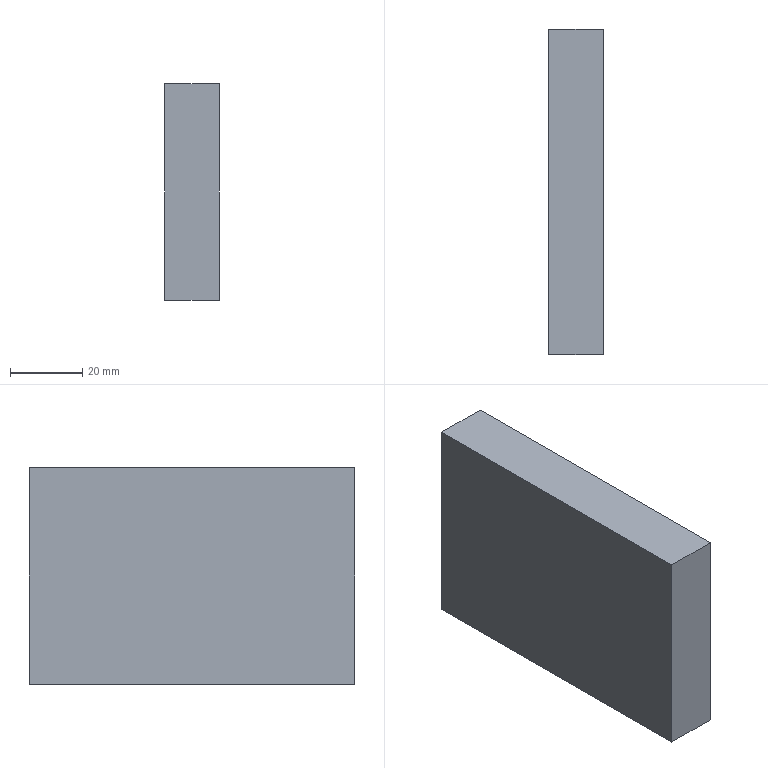Part | STEP file | Tube necking machine_id574_x_t | 1 solid | 6 faces | box 15 x 90 x 60 mm | volume 81000 mm3 | plane 6
STEP:
#1=CARTESIAN_POINT('',(0.,0.,0.));
#2=DIRECTION('',(0.,0.,1.));
#3=DIRECTION('',(1.,0.,0.));
#4=AXIS2_PLACEMENT_3D('',#1,#2,#3);
#5=CARTESIAN_POINT('',(235.5,5.,216.));
#6=VERTEX_POINT('',#5);
#7=CARTESIAN_POINT('',(250.5,5.,216.));
#8=VERTEX_POINT('',#7);
#9=CARTESIAN_POINT('',(235.5,5.,216.));
#10=DIRECTION('',(1.,0.,0.));
#11=VECTOR('',#10,1.);
#12=LINE('',#9,#11);
#13=CARTESIAN_POINT('',(8.,0.,216.));
#14=DIRECTION('',(0.,0.,1.));
#15=DIRECTION('',(1.,0.,0.));
#16=AXIS2_PLACEMENT_3D('',#13,#14,#15);
#17=PLANE('',#16);
#18=CARTESIAN_POINT('',(227.5,5.));
#19=DIRECTION('',(1.,0.));
#20=VECTOR('',#19,1.);
#21=LINE('',#18,#20);
#22=(GEOMETRIC_REPRESENTATION_CONTEXT(2)PARAMETRIC_REPRESENTATION_CONTEXT()REPRESENTATION_CONTEXT('',''));
#23=DEFINITIONAL_REPRESENTATION('',(#21),#22);
#24=PCURVE('',#17,#23);
#25=CARTESIAN_POINT('',(235.5,5.,252.));
#26=DIRECTION('',(0.,1.,0.));
#27=DIRECTION('',(0.,0.,1.));
#28=AXIS2_PLACEMENT_3D('',#25,#26,#27);
#29=PLANE('',#28);
#30=CARTESIAN_POINT('',(-36.,0.));
#31=DIRECTION('',(0.,1.));
#32=VECTOR('',#31,1.);
#33=LINE('',#30,#32);
#34=(GEOMETRIC_REPRESENTATION_CONTEXT(2)PARAMETRIC_REPRESENTATION_CONTEXT()REPRESENTATION_CONTEXT('',''));
#35=DEFINITIONAL_REPRESENTATION('',(#33),#34);
#36=PCURVE('',#29,#35);
#37=SURFACE_CURVE('',#12,(#24,#36),.PCURVE_S1.);
#38=EDGE_CURVE('',#6,#8,#37,.T.);
#39=ORIENTED_EDGE('',*,*,#38,.T.);
#40=CARTESIAN_POINT('',(250.5,95.,216.));
#41=VERTEX_POINT('',#40);
#42=CARTESIAN_POINT('',(250.5,0.,216.));
#43=DIRECTION('',(0.,-1.,0.));
#44=VECTOR('',#43,1.);
#45=LINE('',#42,#44);
#46=CARTESIAN_POINT('',(242.5,0.));
#47=DIRECTION('',(0.,-1.));
#48=VECTOR('',#47,1.);
#49=LINE('',#46,#48);
#50=(GEOMETRIC_REPRESENTATION_CONTEXT(2)PARAMETRIC_REPRESENTATION_CONTEXT()REPRESENTATION_CONTEXT('',''));
#51=DEFINITIONAL_REPRESENTATION('',(#49),#50);
#52=PCURVE('',#17,#51);
#53=CARTESIAN_POINT('',(250.5,80.,332.));
#54=DIRECTION('',(1.,0.,0.));
#55=DIRECTION('',(0.,0.,-1.));
#56=AXIS2_PLACEMENT_3D('',#53,#54,#55);
#57=PLANE('',#56);
#58=CARTESIAN_POINT('',(116.,-80.));
#59=DIRECTION('',(0.,-1.));
#60=VECTOR('',#59,1.);
#61=LINE('',#58,#60);
#62=(GEOMETRIC_REPRESENTATION_CONTEXT(2)PARAMETRIC_REPRESENTATION_CONTEXT()REPRESENTATION_CONTEXT('',''));
#63=DEFINITIONAL_REPRESENTATION('',(#61),#62);
#64=PCURVE('',#57,#63);
#65=SURFACE_CURVE('',#45,(#52,#64),.PCURVE_S1.);
#66=EDGE_CURVE('',#41,#8,#65,.T.);
#67=ORIENTED_EDGE('',*,*,#66,.F.);
#68=CARTESIAN_POINT('',(235.5,95.,216.));
#69=VERTEX_POINT('',#68);
#70=CARTESIAN_POINT('',(305.5,95.,216.));
#71=DIRECTION('',(-1.,0.,0.));
#72=VECTOR('',#71,1.);
#73=LINE('',#70,#72);
#74=CARTESIAN_POINT('',(297.5,95.));
#75=DIRECTION('',(-1.,0.));
#76=VECTOR('',#75,1.);
#77=LINE('',#74,#76);
#78=(GEOMETRIC_REPRESENTATION_CONTEXT(2)PARAMETRIC_REPRESENTATION_CONTEXT()REPRESENTATION_CONTEXT('',''));
#79=DEFINITIONAL_REPRESENTATION('',(#77),#78);
#80=PCURVE('',#17,#79);
#81=CARTESIAN_POINT('',(305.5,95.,252.));
#82=DIRECTION('',(0.,-1.,0.));
#83=DIRECTION('',(0.,0.,-1.));
#84=AXIS2_PLACEMENT_3D('',#81,#82,#83);
#85=PLANE('',#84);
#86=CARTESIAN_POINT('',(36.,0.));
#87=DIRECTION('',(0.,-1.));
#88=VECTOR('',#87,1.);
#89=LINE('',#86,#88);
#90=(GEOMETRIC_REPRESENTATION_CONTEXT(2)PARAMETRIC_REPRESENTATION_CONTEXT()REPRESENTATION_CONTEXT('',''));
#91=DEFINITIONAL_REPRESENTATION('',(#89),#90);
#92=PCURVE('',#85,#91);
#93=SURFACE_CURVE('',#73,(#80,#92),.PCURVE_S1.);
#94=EDGE_CURVE('',#41,#69,#93,.T.);
#95=ORIENTED_EDGE('',*,*,#94,.T.);
#96=CARTESIAN_POINT('',(235.5,95.,216.));
#97=DIRECTION('',(0.,-1.,0.));
#98=VECTOR('',#97,1.);
#99=LINE('',#96,#98);
#100=CARTESIAN_POINT('',(227.5,95.));
#101=DIRECTION('',(0.,-1.));
#102=VECTOR('',#101,1.);
#103=LINE('',#100,#102);
#104=(GEOMETRIC_REPRESENTATION_CONTEXT(2)PARAMETRIC_REPRESENTATION_CONTEXT()REPRESENTATION_CONTEXT('',''));
#105=DEFINITIONAL_REPRESENTATION('',(#103),#104);
#106=PCURVE('',#17,#105);
#107=CARTESIAN_POINT('',(235.5,95.,252.));
#108=DIRECTION('',(1.,0.,0.));
#109=DIRECTION('',(0.,0.,-1.));
#110=AXIS2_PLACEMENT_3D('',#107,#108,#109);
#111=PLANE('',#110);
#112=CARTESIAN_POINT('',(36.,0.));
#113=DIRECTION('',(0.,-1.));
#114=VECTOR('',#113,1.);
#115=LINE('',#112,#114);
#116=(GEOMETRIC_REPRESENTATION_CONTEXT(2)PARAMETRIC_REPRESENTATION_CONTEXT()REPRESENTATION_CONTEXT('',''));
#117=DEFINITIONAL_REPRESENTATION('',(#115),#116);
#118=PCURVE('',#111,#117);
#119=SURFACE_CURVE('',#99,(#106,#118),.PCURVE_S1.);
#120=EDGE_CURVE('',#69,#6,#119,.T.);
#121=ORIENTED_EDGE('',*,*,#120,.T.);
#122=EDGE_LOOP('',(#39,#67,#95,#121));
#123=FACE_BOUND('',#122,.T.);
#124=ADVANCED_FACE('',(#123),#17,.T.);
#125=CARTESIAN_POINT('',(250.5,95.,156.));
#126=VERTEX_POINT('',#125);
#127=CARTESIAN_POINT('',(250.5,5.,156.));
#128=VERTEX_POINT('',#127);
#129=CARTESIAN_POINT('',(250.5,0.,156.));
#130=DIRECTION('',(0.,-1.,0.));
#131=VECTOR('',#130,1.);
#132=LINE('',#129,#131);
#133=CARTESIAN_POINT('',(8.,0.,156.));
#134=DIRECTION('',(0.,0.,1.));
#135=DIRECTION('',(1.,0.,0.));
#136=AXIS2_PLACEMENT_3D('',#133,#134,#135);
#137=PLANE('',#136);
#138=CARTESIAN_POINT('',(242.5,0.));
#139=DIRECTION('',(0.,-1.));
#140=VECTOR('',#139,1.);
#141=LINE('',#138,#140);
#142=(GEOMETRIC_REPRESENTATION_CONTEXT(2)PARAMETRIC_REPRESENTATION_CONTEXT()REPRESENTATION_CONTEXT('',''));
#143=DEFINITIONAL_REPRESENTATION('',(#141),#142);
#144=PCURVE('',#137,#143);
#145=CARTESIAN_POINT('',(176.,-80.));
#146=DIRECTION('',(0.,-1.));
#147=VECTOR('',#146,1.);
#148=LINE('',#145,#147);
#149=(GEOMETRIC_REPRESENTATION_CONTEXT(2)PARAMETRIC_REPRESENTATION_CONTEXT()REPRESENTATION_CONTEXT('',''));
#150=DEFINITIONAL_REPRESENTATION('',(#148),#149);
#151=PCURVE('',#57,#150);
#152=SURFACE_CURVE('',#132,(#144,#151),.PCURVE_S1.);
#153=EDGE_CURVE('',#126,#128,#152,.T.);
#154=ORIENTED_EDGE('',*,*,#153,.T.);
#155=CARTESIAN_POINT('',(235.5,5.,156.));
#156=VERTEX_POINT('',#155);
#157=CARTESIAN_POINT('',(235.5,5.,156.));
#158=DIRECTION('',(1.,0.,0.));
#159=VECTOR('',#158,1.);
#160=LINE('',#157,#159);
#161=CARTESIAN_POINT('',(227.5,5.));
#162=DIRECTION('',(1.,0.));
#163=VECTOR('',#162,1.);
#164=LINE('',#161,#163);
#165=(GEOMETRIC_REPRESENTATION_CONTEXT(2)PARAMETRIC_REPRESENTATION_CONTEXT()REPRESENTATION_CONTEXT('',''));
#166=DEFINITIONAL_REPRESENTATION('',(#164),#165);
#167=PCURVE('',#137,#166);
#168=CARTESIAN_POINT('',(-96.,0.));
#169=DIRECTION('',(0.,1.));
#170=VECTOR('',#169,1.);
#171=LINE('',#168,#170);
#172=(GEOMETRIC_REPRESENTATION_CONTEXT(2)PARAMETRIC_REPRESENTATION_CONTEXT()REPRESENTATION_CONTEXT('',''));
#173=DEFINITIONAL_REPRESENTATION('',(#171),#172);
#174=PCURVE('',#29,#173);
#175=SURFACE_CURVE('',#160,(#167,#174),.PCURVE_S1.);
#176=EDGE_CURVE('',#156,#128,#175,.T.);
#177=ORIENTED_EDGE('',*,*,#176,.F.);
#178=CARTESIAN_POINT('',(235.5,95.,156.));
#179=VERTEX_POINT('',#178);
#180=CARTESIAN_POINT('',(235.5,95.,156.));
#181=DIRECTION('',(0.,-1.,0.));
#182=VECTOR('',#181,1.);
#183=LINE('',#180,#182);
#184=CARTESIAN_POINT('',(227.5,95.));
#185=DIRECTION('',(0.,-1.));
#186=VECTOR('',#185,1.);
#187=LINE('',#184,#186);
#188=(GEOMETRIC_REPRESENTATION_CONTEXT(2)PARAMETRIC_REPRESENTATION_CONTEXT()REPRESENTATION_CONTEXT('',''));
#189=DEFINITIONAL_REPRESENTATION('',(#187),#188);
#190=PCURVE('',#137,#189);
#191=CARTESIAN_POINT('',(96.,0.));
#192=DIRECTION('',(0.,-1.));
#193=VECTOR('',#192,1.);
#194=LINE('',#191,#193);
#195=(GEOMETRIC_REPRESENTATION_CONTEXT(2)PARAMETRIC_REPRESENTATION_CONTEXT()REPRESENTATION_CONTEXT('',''));
#196=DEFINITIONAL_REPRESENTATION('',(#194),#195);
#197=PCURVE('',#111,#196);
#198=SURFACE_CURVE('',#183,(#190,#197),.PCURVE_S1.);
#199=EDGE_CURVE('',#179,#156,#198,.T.);
#200=ORIENTED_EDGE('',*,*,#199,.F.);
#201=CARTESIAN_POINT('',(305.5,95.,156.));
#202=DIRECTION('',(-1.,0.,0.));
#203=VECTOR('',#202,1.);
#204=LINE('',#201,#203);
#205=CARTESIAN_POINT('',(297.5,95.));
#206=DIRECTION('',(-1.,0.));
#207=VECTOR('',#206,1.);
#208=LINE('',#205,#207);
#209=(GEOMETRIC_REPRESENTATION_CONTEXT(2)PARAMETRIC_REPRESENTATION_CONTEXT()REPRESENTATION_CONTEXT('',''));
#210=DEFINITIONAL_REPRESENTATION('',(#208),#209);
#211=PCURVE('',#137,#210);
#212=CARTESIAN_POINT('',(96.,0.));
#213=DIRECTION('',(0.,-1.));
#214=VECTOR('',#213,1.);
#215=LINE('',#212,#214);
#216=(GEOMETRIC_REPRESENTATION_CONTEXT(2)PARAMETRIC_REPRESENTATION_CONTEXT()REPRESENTATION_CONTEXT('',''));
#217=DEFINITIONAL_REPRESENTATION('',(#215),#216);
#218=PCURVE('',#85,#217);
#219=SURFACE_CURVE('',#204,(#211,#218),.PCURVE_S1.);
#220=EDGE_CURVE('',#126,#179,#219,.T.);
#221=ORIENTED_EDGE('',*,*,#220,.F.);
#222=EDGE_LOOP('',(#154,#177,#200,#221));
#223=FACE_BOUND('',#222,.T.);
#224=ADVANCED_FACE('',(#223),#137,.F.);
#225=CARTESIAN_POINT('',(250.5,5.,252.));
#226=DIRECTION('',(0.,0.,-1.));
#227=VECTOR('',#226,1.);
#228=LINE('',#225,#227);
#229=CARTESIAN_POINT('',(0.,15.));
#230=DIRECTION('',(-1.,0.));
#231=VECTOR('',#230,1.);
#232=LINE('',#229,#231);
#233=(GEOMETRIC_REPRESENTATION_CONTEXT(2)PARAMETRIC_REPRESENTATION_CONTEXT()REPRESENTATION_CONTEXT('',''));
#234=DEFINITIONAL_REPRESENTATION('',(#232),#233);
#235=PCURVE('',#29,#234);
#236=CARTESIAN_POINT('',(80.,-75.));
#237=DIRECTION('',(1.,0.));
#238=VECTOR('',#237,1.);
#239=LINE('',#236,#238);
#240=(GEOMETRIC_REPRESENTATION_CONTEXT(2)PARAMETRIC_REPRESENTATION_CONTEXT()REPRESENTATION_CONTEXT('',''));
#241=DEFINITIONAL_REPRESENTATION('',(#239),#240);
#242=PCURVE('',#57,#241);
#243=SURFACE_CURVE('',#228,(#235,#242),.PCURVE_S1.);
#244=EDGE_CURVE('',#8,#128,#243,.T.);
#245=ORIENTED_EDGE('',*,*,#244,.F.);
#246=ORIENTED_EDGE('',*,*,#38,.F.);
#247=CARTESIAN_POINT('',(235.5,5.,252.));
#248=DIRECTION('',(0.,0.,-1.));
#249=VECTOR('',#248,1.);
#250=LINE('',#247,#249);
#251=CARTESIAN_POINT('',(0.,0.));
#252=DIRECTION('',(-1.,0.));
#253=VECTOR('',#252,1.);
#254=LINE('',#251,#253);
#255=(GEOMETRIC_REPRESENTATION_CONTEXT(2)PARAMETRIC_REPRESENTATION_CONTEXT()REPRESENTATION_CONTEXT('',''));
#256=DEFINITIONAL_REPRESENTATION('',(#254),#255);
#257=PCURVE('',#29,#256);
#258=CARTESIAN_POINT('',(0.,-90.));
#259=DIRECTION('',(1.,0.));
#260=VECTOR('',#259,1.);
#261=LINE('',#258,#260);
#262=(GEOMETRIC_REPRESENTATION_CONTEXT(2)PARAMETRIC_REPRESENTATION_CONTEXT()REPRESENTATION_CONTEXT('',''));
#263=DEFINITIONAL_REPRESENTATION('',(#261),#262);
#264=PCURVE('',#111,#263);
#265=SURFACE_CURVE('',#250,(#257,#264),.PCURVE_S1.);
#266=EDGE_CURVE('',#6,#156,#265,.T.);
#267=ORIENTED_EDGE('',*,*,#266,.T.);
#268=ORIENTED_EDGE('',*,*,#176,.T.);
#269=EDGE_LOOP('',(#245,#246,#267,#268));
#270=FACE_BOUND('',#269,.T.);
#271=ADVANCED_FACE('',(#270),#29,.F.);
#272=CARTESIAN_POINT('',(250.5,95.,252.));
#273=DIRECTION('',(0.,0.,1.));
#274=VECTOR('',#273,1.);
#275=LINE('',#272,#274);
#276=CARTESIAN_POINT('',(0.,-55.));
#277=DIRECTION('',(-1.,0.));
#278=VECTOR('',#277,1.);
#279=LINE('',#276,#278);
#280=(GEOMETRIC_REPRESENTATION_CONTEXT(2)PARAMETRIC_REPRESENTATION_CONTEXT()REPRESENTATION_CONTEXT('',''));
#281=DEFINITIONAL_REPRESENTATION('',(#279),#280);
#282=PCURVE('',#85,#281);
#283=CARTESIAN_POINT('',(80.,15.));
#284=DIRECTION('',(-1.,0.));
#285=VECTOR('',#284,1.);
#286=LINE('',#283,#285);
#287=(GEOMETRIC_REPRESENTATION_CONTEXT(2)PARAMETRIC_REPRESENTATION_CONTEXT()REPRESENTATION_CONTEXT('',''));
#288=DEFINITIONAL_REPRESENTATION('',(#286),#287);
#289=PCURVE('',#57,#288);
#290=SURFACE_CURVE('',#275,(#282,#289),.PCURVE_S1.);
#291=EDGE_CURVE('',#126,#41,#290,.T.);
#292=ORIENTED_EDGE('',*,*,#291,.F.);
#293=ORIENTED_EDGE('',*,*,#220,.T.);
#294=CARTESIAN_POINT('',(235.5,95.,252.));
#295=DIRECTION('',(0.,0.,-1.));
#296=VECTOR('',#295,1.);
#297=LINE('',#294,#296);
#298=CARTESIAN_POINT('',(0.,-70.));
#299=DIRECTION('',(1.,0.));
#300=VECTOR('',#299,1.);
#301=LINE('',#298,#300);
#302=(GEOMETRIC_REPRESENTATION_CONTEXT(2)PARAMETRIC_REPRESENTATION_CONTEXT()REPRESENTATION_CONTEXT('',''));
#303=DEFINITIONAL_REPRESENTATION('',(#301),#302);
#304=PCURVE('',#85,#303);
#305=CARTESIAN_POINT('',(0.,0.));
#306=DIRECTION('',(1.,0.));
#307=VECTOR('',#306,1.);
#308=LINE('',#305,#307);
#309=(GEOMETRIC_REPRESENTATION_CONTEXT(2)PARAMETRIC_REPRESENTATION_CONTEXT()REPRESENTATION_CONTEXT('',''));
#310=DEFINITIONAL_REPRESENTATION('',(#308),#309);
#311=PCURVE('',#111,#310);
#312=SURFACE_CURVE('',#297,(#304,#311),.PCURVE_S1.);
#313=EDGE_CURVE('',#69,#179,#312,.T.);
#314=ORIENTED_EDGE('',*,*,#313,.F.);
#315=ORIENTED_EDGE('',*,*,#94,.F.);
#316=EDGE_LOOP('',(#292,#293,#314,#315));
#317=FACE_BOUND('',#316,.T.);
#318=ADVANCED_FACE('',(#317),#85,.F.);
#319=ORIENTED_EDGE('',*,*,#199,.T.);
#320=ORIENTED_EDGE('',*,*,#266,.F.);
#321=ORIENTED_EDGE('',*,*,#120,.F.);
#322=ORIENTED_EDGE('',*,*,#313,.T.);
#323=EDGE_LOOP('',(#319,#320,#321,#322));
#324=FACE_BOUND('',#323,.T.);
#325=ADVANCED_FACE('',(#324),#111,.F.);
#326=ORIENTED_EDGE('',*,*,#291,.T.);
#327=ORIENTED_EDGE('',*,*,#66,.T.);
#328=ORIENTED_EDGE('',*,*,#244,.T.);
#329=ORIENTED_EDGE('',*,*,#153,.F.);
#330=EDGE_LOOP('',(#326,#327,#328,#329));
#331=FACE_BOUND('',#330,.T.);
#332=ADVANCED_FACE('',(#331),#57,.T.);
#333=CLOSED_SHELL('',(#124,#224,#271,#318,#325,#332));
#334=MANIFOLD_SOLID_BREP('',#333);
#335=(LENGTH_UNIT()NAMED_UNIT(*)SI_UNIT(.MILLI.,.METRE.));
#336=UNCERTAINTY_MEASURE_WITH_UNIT(LENGTH_MEASURE(0.0000001),#335,'','');
#337=(NAMED_UNIT(*)PLANE_ANGLE_UNIT()SI_UNIT($,.RADIAN.));
#338=(NAMED_UNIT(*)SI_UNIT($,.STERADIAN.)SOLID_ANGLE_UNIT());
#339=(GEOMETRIC_REPRESENTATION_CONTEXT(3)GLOBAL_UNCERTAINTY_ASSIGNED_CONTEXT((#336))GLOBAL_UNIT_ASSIGNED_CONTEXT((#335,#337,#338))REPRESENTATION_CONTEXT('',''));
#340=ADVANCED_BREP_SHAPE_REPRESENTATION('',(#4,#334),#339);